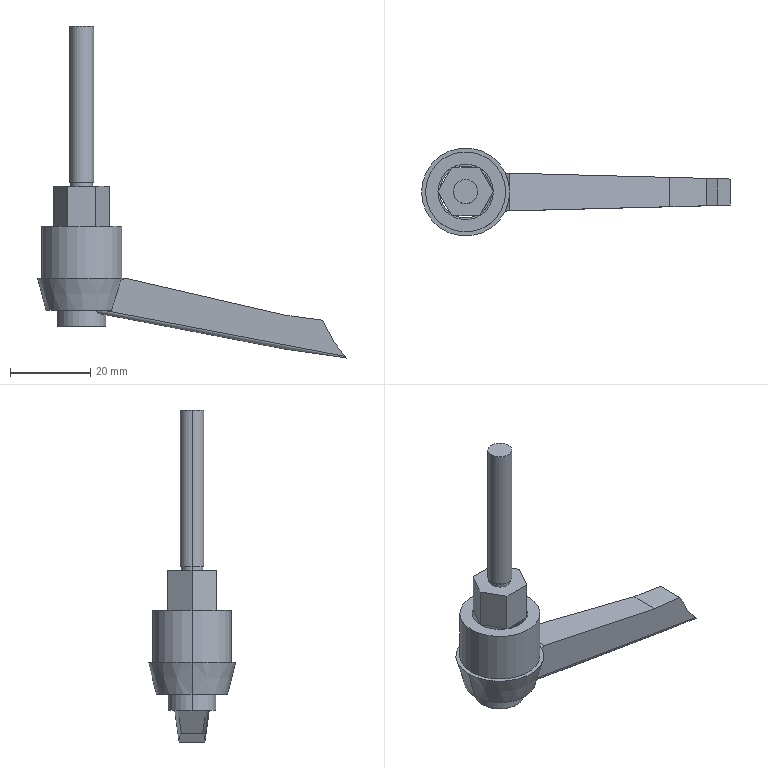Part | STEP file | M8 M6 M102(M6_45_40) | 2 solids | 60 faces | box 77.136 x 22 x 82.928 mm | volume 11260 mm3 | plane 44 | cylinder 14 | cone 2 | commonest cylinder face diameters 2 x2 5.5 x2 6 x2 12 x2 13 x2 13.856 x2